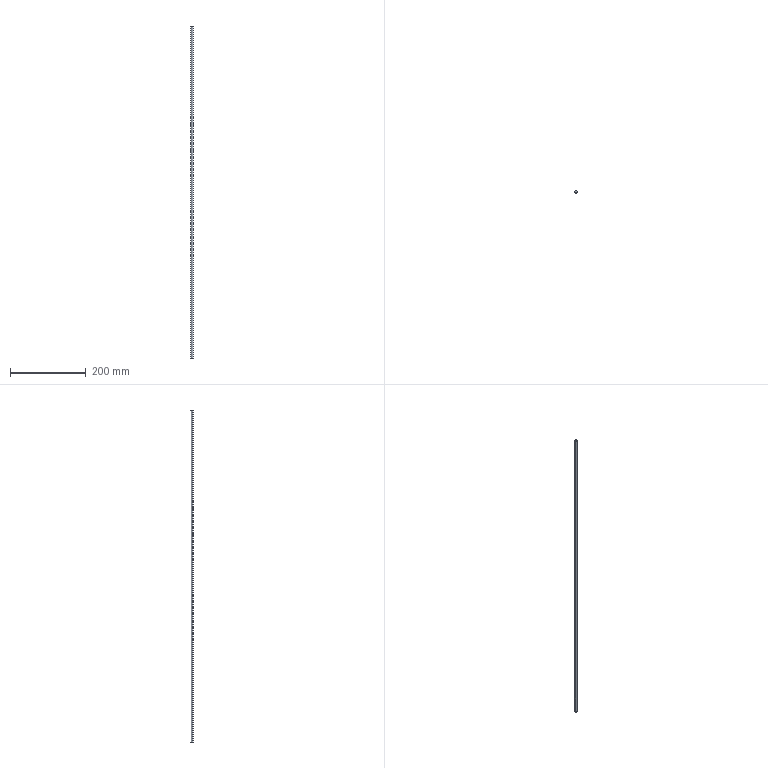Part | SolidWorks | features Extrusion 1 | 1 solid | 4 faces | box 6 x 6 x 875 mm | volume 24740 mm3 | cylinder 2 | plane 2 | commonest cylinder face diameters 6 x2
STEP:
#1=CARTESIAN_POINT('',(3.,0.,875.));
#2=VERTEX_POINT('',#1);
#3=CARTESIAN_POINT('',(-3.,0.,875.));
#4=VERTEX_POINT('',#3);
#5=CARTESIAN_POINT('',(0.,0.,875.));
#6=DIRECTION('',(0.,0.,1.));
#7=DIRECTION('',(1.,0.,0.));
#8=AXIS2_PLACEMENT_3D('',#5,#6,#7);
#9=CIRCLE('',#8,3.);
#10=EDGE_CURVE('',#2,#4,#9,.T.);
#11=ORIENTED_EDGE('',*,*,#10,.F.);
#12=CARTESIAN_POINT('',(3.,0.,0.));
#13=VERTEX_POINT('',#12);
#14=CARTESIAN_POINT('',(3.,0.,875.));
#15=DIRECTION('',(0.,0.,-1.));
#16=VECTOR('',#15,1000.);
#17=LINE('',#14,#16);
#18=EDGE_CURVE('',#2,#13,#17,.T.);
#19=ORIENTED_EDGE('',*,*,#18,.T.);
#20=CARTESIAN_POINT('',(-3.,0.,0.));
#21=VERTEX_POINT('',#20);
#22=CARTESIAN_POINT('',(0.,0.,0.));
#23=DIRECTION('',(0.,0.,1.));
#24=DIRECTION('',(1.,0.,0.));
#25=AXIS2_PLACEMENT_3D('',#22,#23,#24);
#26=CIRCLE('',#25,3.);
#27=EDGE_CURVE('',#13,#21,#26,.T.);
#28=ORIENTED_EDGE('',*,*,#27,.T.);
#29=CARTESIAN_POINT('',(-3.,0.,875.));
#30=DIRECTION('',(0.,0.,-1.));
#31=VECTOR('',#30,1000.);
#32=LINE('',#29,#31);
#33=EDGE_CURVE('',#4,#21,#32,.T.);
#34=ORIENTED_EDGE('',*,*,#33,.F.);
#35=EDGE_LOOP('',(#11,#19,#28,#34));
#36=FACE_OUTER_BOUND('',#35,.T.);
#37=CARTESIAN_POINT('',(0.,0.,875.));
#38=DIRECTION('',(0.,0.,-1.));
#39=DIRECTION('',(-1.,0.,0.));
#40=AXIS2_PLACEMENT_3D('',#37,#38,#39);
#41=CYLINDRICAL_SURFACE('',#40,3.);
#42=ADVANCED_FACE('',(#36),#41,.T.);
#43=ORIENTED_EDGE('',*,*,#18,.F.);
#44=CARTESIAN_POINT('',(0.,0.,875.));
#45=DIRECTION('',(0.,0.,1.));
#46=DIRECTION('',(1.,0.,0.));
#47=AXIS2_PLACEMENT_3D('',#44,#45,#46);
#48=CIRCLE('',#47,3.);
#49=EDGE_CURVE('',#4,#2,#48,.T.);
#50=ORIENTED_EDGE('',*,*,#49,.F.);
#51=ORIENTED_EDGE('',*,*,#33,.T.);
#52=CARTESIAN_POINT('',(0.,0.,0.));
#53=DIRECTION('',(0.,0.,1.));
#54=DIRECTION('',(1.,0.,0.));
#55=AXIS2_PLACEMENT_3D('',#52,#53,#54);
#56=CIRCLE('',#55,3.);
#57=EDGE_CURVE('',#21,#13,#56,.T.);
#58=ORIENTED_EDGE('',*,*,#57,.T.);
#59=EDGE_LOOP('',(#43,#50,#51,#58));
#60=FACE_OUTER_BOUND('',#59,.T.);
#61=CARTESIAN_POINT('',(0.,0.,875.));
#62=DIRECTION('',(0.,0.,-1.));
#63=DIRECTION('',(-1.,0.,0.));
#64=AXIS2_PLACEMENT_3D('',#61,#62,#63);
#65=CYLINDRICAL_SURFACE('',#64,3.);
#66=ADVANCED_FACE('',(#60),#65,.T.);
#67=ORIENTED_EDGE('',*,*,#49,.T.);
#68=ORIENTED_EDGE('',*,*,#10,.T.);
#69=EDGE_LOOP('',(#67,#68));
#70=FACE_OUTER_BOUND('',#69,.T.);
#71=CARTESIAN_POINT('',(0.,0.,875.));
#72=DIRECTION('',(0.,0.,1.));
#73=DIRECTION('',(1.,0.,0.));
#74=AXIS2_PLACEMENT_3D('',#71,#72,#73);
#75=PLANE('',#74);
#76=ADVANCED_FACE('',(#70),#75,.T.);
#77=ORIENTED_EDGE('',*,*,#57,.F.);
#78=ORIENTED_EDGE('',*,*,#27,.F.);
#79=EDGE_LOOP('',(#77,#78));
#80=FACE_OUTER_BOUND('',#79,.T.);
#81=CARTESIAN_POINT('',(0.,0.,0.));
#82=DIRECTION('',(0.,0.,1.));
#83=DIRECTION('',(1.,0.,0.));
#84=AXIS2_PLACEMENT_3D('',#81,#82,#83);
#85=PLANE('',#84);
#86=ADVANCED_FACE('',(#80),#85,.F.);
#87=CLOSED_SHELL('',(#42,#66,#76,#86));
#88=MANIFOLD_SOLID_BREP('',#87);
#89=CARTESIAN_POINT('',(0.,0.,0.));
#90=DIRECTION('',(0.,0.,1.));
#91=DIRECTION('',(1.,0.,0.));
#92=AXIS2_PLACEMENT_3D('',#89,#90,#91);
#93=(LENGTH_UNIT()NAMED_UNIT(*)SI_UNIT(.MILLI.,.METRE.));
#94=UNCERTAINTY_MEASURE_WITH_UNIT(LENGTH_MEASURE(0.00001),#93,'','');
#95=(NAMED_UNIT(*)PLANE_ANGLE_UNIT()SI_UNIT($,.RADIAN.));
#96=(NAMED_UNIT(*)SI_UNIT($,.STERADIAN.)SOLID_ANGLE_UNIT());
#97=(GEOMETRIC_REPRESENTATION_CONTEXT(3)GLOBAL_UNCERTAINTY_ASSIGNED_CONTEXT((#94))GLOBAL_UNIT_ASSIGNED_CONTEXT((#93,#95,#96))REPRESENTATION_CONTEXT('',''));
#98=ADVANCED_BREP_SHAPE_REPRESENTATION('',(#88,#92),#97);